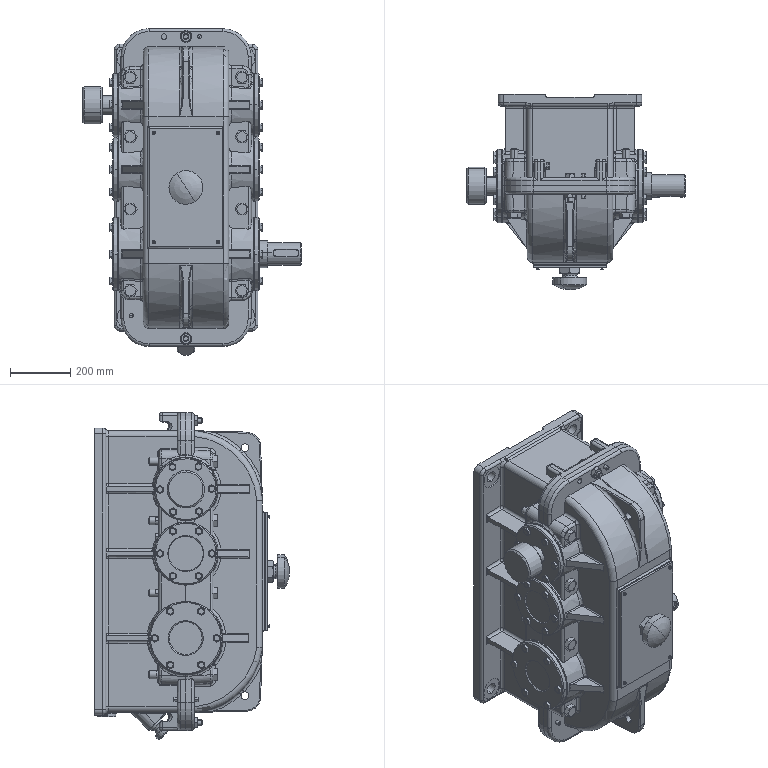Part | SolidWorks | features ReferencePattern 45, CompositeCurve 27, MirrorCompFeat 4, LocalCirPattern 3, AEMSimFeature 1 | 202 solids | 6521 faces | volume 87002106 mm3 | cylinder 2931 | plane 1878 | torus 873 | cone 587 | spline 160 | sphere 92 | commonest cylinder face diameters 15 x290 1.875 x279 88.125 x242 3.75 x223 115.716 x188 143.1 x182